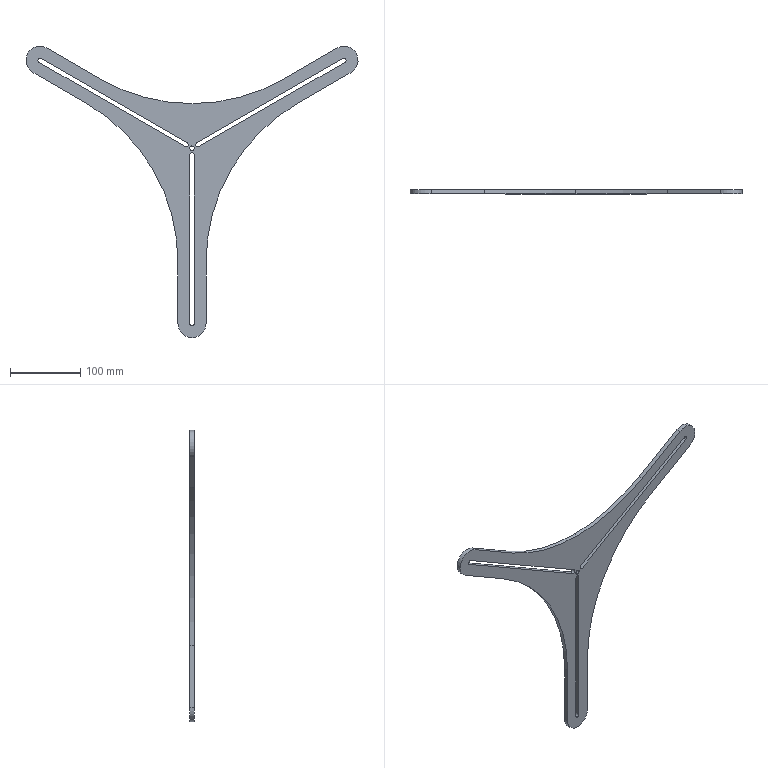Part | SolidWorks | features Extrusion 1 | 1 solid | 33 faces | box 472.147 x 6 x 414.25 mm | volume 225588 mm3 | cylinder 19 | plane 14 | commonest cylinder face diameters 6 x9 40 x4 520 x4 6.2 x2
STEP:
#1=CARTESIAN_POINT('',(15.557,6.,-256.75));
#2=VERTEX_POINT('',#1);
#3=CARTESIAN_POINT('',(12.557,6.,-259.75));
#4=VERTEX_POINT('',#3);
#5=CARTESIAN_POINT('',(12.557,6.,-256.75));
#6=DIRECTION('',(0.,1.,0.));
#7=DIRECTION('',(0.,0.,1.));
#8=AXIS2_PLACEMENT_3D('',#5,#6,#7);
#9=CIRCLE('',#8,3.);
#10=EDGE_CURVE('',#2,#4,#9,.T.);
#11=ORIENTED_EDGE('',*,*,#10,.T.);
#12=CARTESIAN_POINT('',(12.557,0.,-259.75));
#13=VERTEX_POINT('',#12);
#14=CARTESIAN_POINT('',(12.557,6.,-259.75));
#15=DIRECTION('',(0.,-1.,0.));
#16=VECTOR('',#15,1000.);
#17=LINE('',#14,#16);
#18=EDGE_CURVE('',#4,#13,#17,.T.);
#19=ORIENTED_EDGE('',*,*,#18,.T.);
#20=CARTESIAN_POINT('',(15.557,0.,-256.75));
#21=VERTEX_POINT('',#20);
#22=CARTESIAN_POINT('',(12.557,0.,-256.75));
#23=DIRECTION('',(0.,1.,0.));
#24=DIRECTION('',(0.,0.,1.));
#25=AXIS2_PLACEMENT_3D('',#22,#23,#24);
#26=CIRCLE('',#25,3.);
#27=EDGE_CURVE('',#21,#13,#26,.T.);
#28=ORIENTED_EDGE('',*,*,#27,.F.);
#29=CARTESIAN_POINT('',(15.557,6.,-256.75));
#30=DIRECTION('',(0.,-1.,0.));
#31=VECTOR('',#30,1000.);
#32=LINE('',#29,#31);
#33=EDGE_CURVE('',#2,#21,#32,.T.);
#34=ORIENTED_EDGE('',*,*,#33,.F.);
#35=EDGE_LOOP('',(#11,#19,#28,#34));
#36=FACE_OUTER_BOUND('',#35,.T.);
#37=CARTESIAN_POINT('',(12.557,6.,-256.75));
#38=DIRECTION('',(0.,-1.,0.));
#39=DIRECTION('',(0.,0.,-1.));
#40=AXIS2_PLACEMENT_3D('',#37,#38,#39);
#41=CYLINDRICAL_SURFACE('',#40,3.);
#42=ADVANCED_FACE('',(#36),#41,.F.);
#43=CARTESIAN_POINT('',(22.285,6.,-5.098));
#44=VERTEX_POINT('',#43);
#45=CARTESIAN_POINT('',(20.785,6.,-5.5));
#46=VERTEX_POINT('',#45);
#47=CARTESIAN_POINT('',(20.785,6.,-2.5));
#48=DIRECTION('',(0.,1.,0.));
#49=DIRECTION('',(0.,0.,1.));
#50=AXIS2_PLACEMENT_3D('',#47,#48,#49);
#51=CIRCLE('',#50,3.);
#52=EDGE_CURVE('',#44,#46,#51,.T.);
#53=ORIENTED_EDGE('',*,*,#52,.T.);
#54=CARTESIAN_POINT('',(20.785,0.,-5.5));
#55=VERTEX_POINT('',#54);
#56=CARTESIAN_POINT('',(20.785,6.,-5.5));
#57=DIRECTION('',(0.,-1.,0.));
#58=VECTOR('',#57,1000.);
#59=LINE('',#56,#58);
#60=EDGE_CURVE('',#46,#55,#59,.T.);
#61=ORIENTED_EDGE('',*,*,#60,.T.);
#62=CARTESIAN_POINT('',(22.285,0.,-5.098));
#63=VERTEX_POINT('',#62);
#64=CARTESIAN_POINT('',(20.785,0.,-2.5));
#65=DIRECTION('',(0.,1.,0.));
#66=DIRECTION('',(0.,0.,1.));
#67=AXIS2_PLACEMENT_3D('',#64,#65,#66);
#68=CIRCLE('',#67,3.);
#69=EDGE_CURVE('',#63,#55,#68,.T.);
#70=ORIENTED_EDGE('',*,*,#69,.F.);
#71=CARTESIAN_POINT('',(22.285,6.,-5.098));
#72=DIRECTION('',(0.,-1.,0.));
#73=VECTOR('',#72,1000.);
#74=LINE('',#71,#73);
#75=EDGE_CURVE('',#44,#63,#74,.T.);
#76=ORIENTED_EDGE('',*,*,#75,.F.);
#77=EDGE_LOOP('',(#53,#61,#70,#76));
#78=FACE_OUTER_BOUND('',#77,.T.);
#79=CARTESIAN_POINT('',(20.785,6.,-2.5));
#80=DIRECTION('',(0.,-1.,0.));
#81=DIRECTION('',(0.,0.,-1.));
#82=AXIS2_PLACEMENT_3D('',#79,#80,#81);
#83=CYLINDRICAL_SURFACE('',#82,3.);
#84=ADVANCED_FACE('',(#78),#83,.F.);
#85=CARTESIAN_POINT('',(5.83,6.,0.09808));
#86=VERTEX_POINT('',#85);
#87=CARTESIAN_POINT('',(4.33,6.,-5.5));
#88=VERTEX_POINT('',#87);
#89=CARTESIAN_POINT('',(4.33,6.,-2.5));
#90=DIRECTION('',(0.,1.,0.));
#91=DIRECTION('',(0.,0.,1.));
#92=AXIS2_PLACEMENT_3D('',#89,#90,#91);
#93=CIRCLE('',#92,3.);
#94=EDGE_CURVE('',#86,#88,#93,.T.);
#95=ORIENTED_EDGE('',*,*,#94,.T.);
#96=CARTESIAN_POINT('',(4.33,0.,-5.5));
#97=VERTEX_POINT('',#96);
#98=CARTESIAN_POINT('',(4.33,6.,-5.5));
#99=DIRECTION('',(0.,-1.,0.));
#100=VECTOR('',#99,1000.);
#101=LINE('',#98,#100);
#102=EDGE_CURVE('',#88,#97,#101,.T.);
#103=ORIENTED_EDGE('',*,*,#102,.T.);
#104=CARTESIAN_POINT('',(5.83,0.,0.09808));
#105=VERTEX_POINT('',#104);
#106=CARTESIAN_POINT('',(4.33,0.,-2.5));
#107=DIRECTION('',(0.,1.,0.));
#108=DIRECTION('',(0.,0.,1.));
#109=AXIS2_PLACEMENT_3D('',#106,#107,#108);
#110=CIRCLE('',#109,3.);
#111=EDGE_CURVE('',#105,#97,#110,.T.);
#112=ORIENTED_EDGE('',*,*,#111,.F.);
#113=CARTESIAN_POINT('',(5.83,6.,0.09808));
#114=DIRECTION('',(0.,-1.,0.));
#115=VECTOR('',#114,1000.);
#116=LINE('',#113,#115);
#117=EDGE_CURVE('',#86,#105,#116,.T.);
#118=ORIENTED_EDGE('',*,*,#117,.F.);
#119=EDGE_LOOP('',(#95,#103,#112,#118));
#120=FACE_OUTER_BOUND('',#119,.T.);
#121=CARTESIAN_POINT('',(4.33,6.,-2.5));
#122=DIRECTION('',(0.,-1.,0.));
#123=DIRECTION('',(0.,0.,-1.));
#124=AXIS2_PLACEMENT_3D('',#121,#122,#123);
#125=CYLINDRICAL_SURFACE('',#124,3.);
#126=ADVANCED_FACE('',(#120),#125,.F.);
#127=CARTESIAN_POINT('',(12.557,6.,-10.35));
#128=VERTEX_POINT('',#127);
#129=CARTESIAN_POINT('',(12.557,6.,-4.15));
#130=VERTEX_POINT('',#129);
#131=CARTESIAN_POINT('',(12.557,6.,-7.25));
#132=DIRECTION('',(0.,1.,0.));
#133=DIRECTION('',(0.,0.,1.));
#134=AXIS2_PLACEMENT_3D('',#131,#132,#133);
#135=CIRCLE('',#134,3.1);
#136=EDGE_CURVE('',#128,#130,#135,.T.);
#137=ORIENTED_EDGE('',*,*,#136,.T.);
#138=CARTESIAN_POINT('',(12.557,0.,-4.15));
#139=VERTEX_POINT('',#138);
#140=CARTESIAN_POINT('',(12.557,6.,-4.15));
#141=DIRECTION('',(0.,-1.,0.));
#142=VECTOR('',#141,1000.);
#143=LINE('',#140,#142);
#144=EDGE_CURVE('',#130,#139,#143,.T.);
#145=ORIENTED_EDGE('',*,*,#144,.T.);
#146=CARTESIAN_POINT('',(12.557,0.,-10.35));
#147=VERTEX_POINT('',#146);
#148=CARTESIAN_POINT('',(12.557,0.,-7.25));
#149=DIRECTION('',(0.,1.,0.));
#150=DIRECTION('',(0.,0.,1.));
#151=AXIS2_PLACEMENT_3D('',#148,#149,#150);
#152=CIRCLE('',#151,3.1);
#153=EDGE_CURVE('',#147,#139,#152,.T.);
#154=ORIENTED_EDGE('',*,*,#153,.F.);
#155=CARTESIAN_POINT('',(12.557,6.,-10.35));
#156=DIRECTION('',(0.,-1.,0.));
#157=VECTOR('',#156,1000.);
#158=LINE('',#155,#157);
#159=EDGE_CURVE('',#128,#147,#158,.T.);
#160=ORIENTED_EDGE('',*,*,#159,.F.);
#161=EDGE_LOOP('',(#137,#145,#154,#160));
#162=FACE_OUTER_BOUND('',#161,.T.);
#163=CARTESIAN_POINT('',(12.557,6.,-7.25));
#164=DIRECTION('',(0.,-1.,0.));
#165=DIRECTION('',(0.,0.,-1.));
#166=AXIS2_PLACEMENT_3D('',#163,#164,#165);
#167=CYLINDRICAL_SURFACE('',#166,3.1);
#168=ADVANCED_FACE('',(#162),#167,.F.);
#169=CARTESIAN_POINT('',(12.557,6.,56.066));
#170=VERTEX_POINT('',#169);
#171=CARTESIAN_POINT('',(142.557,6.,90.9));
#172=VERTEX_POINT('',#171);
#173=CARTESIAN_POINT('',(12.557,6.,316.066));
#174=DIRECTION('',(0.,-1.,0.));
#175=DIRECTION('',(0.,0.,-1.));
#176=AXIS2_PLACEMENT_3D('',#173,#174,#175);
#177=CIRCLE('',#176,260.);
#178=EDGE_CURVE('',#170,#172,#177,.T.);
#179=ORIENTED_EDGE('',*,*,#178,.F.);
#180=CARTESIAN_POINT('',(12.557,0.,56.066));
#181=VERTEX_POINT('',#180);
#182=CARTESIAN_POINT('',(12.557,6.,56.066));
#183=DIRECTION('',(0.,-1.,0.));
#184=VECTOR('',#183,1000.);
#185=LINE('',#182,#184);
#186=EDGE_CURVE('',#170,#181,#185,.T.);
#187=ORIENTED_EDGE('',*,*,#186,.T.);
#188=CARTESIAN_POINT('',(142.557,0.,90.9));
#189=VERTEX_POINT('',#188);
#190=CARTESIAN_POINT('',(12.557,0.,316.066));
#191=DIRECTION('',(0.,-1.,0.));
#192=DIRECTION('',(0.,0.,-1.));
#193=AXIS2_PLACEMENT_3D('',#190,#191,#192);
#194=CIRCLE('',#193,260.);
#195=EDGE_CURVE('',#181,#189,#194,.T.);
#196=ORIENTED_EDGE('',*,*,#195,.T.);
#197=CARTESIAN_POINT('',(142.557,6.,90.9));
#198=DIRECTION('',(0.,-1.,0.));
#199=VECTOR('',#198,1000.);
#200=LINE('',#197,#199);
#201=EDGE_CURVE('',#172,#189,#200,.T.);
#202=ORIENTED_EDGE('',*,*,#201,.F.);
#203=EDGE_LOOP('',(#179,#187,#196,#202));
#204=FACE_OUTER_BOUND('',#203,.T.);
#205=CARTESIAN_POINT('',(12.557,6.,316.066));
#206=DIRECTION('',(0.,-1.,0.));
#207=DIRECTION('',(0.,0.,-1.));
#208=AXIS2_PLACEMENT_3D('',#205,#206,#207);
#209=CYLINDRICAL_SURFACE('',#208,260.);
#210=ADVANCED_FACE('',(#204),#209,.F.);
#211=CARTESIAN_POINT('',(12.557,6.,-276.75));
#212=VERTEX_POINT('',#211);
#213=CARTESIAN_POINT('',(-7.443,6.,-256.75));
#214=VERTEX_POINT('',#213);
#215=CARTESIAN_POINT('',(12.557,6.,-256.75));
#216=DIRECTION('',(0.,1.,0.));
#217=DIRECTION('',(0.,0.,-1.));
#218=AXIS2_PLACEMENT_3D('',#215,#216,#217);
#219=CIRCLE('',#218,20.);
#220=EDGE_CURVE('',#212,#214,#219,.T.);
#221=ORIENTED_EDGE('',*,*,#220,.F.);
#222=CARTESIAN_POINT('',(12.557,0.,-276.75));
#223=VERTEX_POINT('',#222);
#224=CARTESIAN_POINT('',(12.557,6.,-276.75));
#225=DIRECTION('',(0.,-1.,0.));
#226=VECTOR('',#225,1000.);
#227=LINE('',#224,#226);
#228=EDGE_CURVE('',#212,#223,#227,.T.);
#229=ORIENTED_EDGE('',*,*,#228,.T.);
#230=CARTESIAN_POINT('',(-7.443,0.,-256.75));
#231=VERTEX_POINT('',#230);
#232=CARTESIAN_POINT('',(12.557,0.,-256.75));
#233=DIRECTION('',(0.,1.,0.));
#234=DIRECTION('',(0.,0.,-1.));
#235=AXIS2_PLACEMENT_3D('',#232,#233,#234);
#236=CIRCLE('',#235,20.);
#237=EDGE_CURVE('',#223,#231,#236,.T.);
#238=ORIENTED_EDGE('',*,*,#237,.T.);
#239=CARTESIAN_POINT('',(-7.443,6.,-256.75));
#240=DIRECTION('',(0.,-1.,0.));
#241=VECTOR('',#240,1000.);
#242=LINE('',#239,#241);
#243=EDGE_CURVE('',#214,#231,#242,.T.);
#244=ORIENTED_EDGE('',*,*,#243,.F.);
#245=EDGE_LOOP('',(#221,#229,#238,#244));
#246=FACE_OUTER_BOUND('',#245,.T.);
#247=CARTESIAN_POINT('',(12.557,6.,-256.75));
#248=DIRECTION('',(0.,-1.,0.));
#249=DIRECTION('',(0.,0.,-1.));
#250=AXIS2_PLACEMENT_3D('',#247,#248,#249);
#251=CYLINDRICAL_SURFACE('',#250,20.);
#252=ADVANCED_FACE('',(#246),#251,.T.);
#253=ORIENTED_EDGE('',*,*,#52,.F.);
#254=CARTESIAN_POINT('',(230.131,6.,114.902));
#255=VERTEX_POINT('',#254);
#256=CARTESIAN_POINT('',(22.285,6.,-5.098));
#257=DIRECTION('',(-0.866,0.,-0.5));
#258=VECTOR('',#257,1000.);
#259=LINE('',#256,#258);
#260=EDGE_CURVE('',#255,#44,#259,.T.);
#261=ORIENTED_EDGE('',*,*,#260,.F.);
#262=CARTESIAN_POINT('',(227.131,6.,120.098));
#263=VERTEX_POINT('',#262);
#264=CARTESIAN_POINT('',(228.631,6.,117.5));
#265=DIRECTION('',(0.,1.,0.));
#266=DIRECTION('',(0.,0.,1.));
#267=AXIS2_PLACEMENT_3D('',#264,#265,#266);
#268=CIRCLE('',#267,3.);
#269=EDGE_CURVE('',#263,#255,#268,.T.);
#270=ORIENTED_EDGE('',*,*,#269,.F.);
#271=CARTESIAN_POINT('',(19.285,6.,0.09808));
#272=VERTEX_POINT('',#271);
#273=CARTESIAN_POINT('',(19.285,6.,0.09808));
#274=DIRECTION('',(0.866,0.,0.5));
#275=VECTOR('',#274,1000.);
#276=LINE('',#273,#275);
#277=EDGE_CURVE('',#272,#263,#276,.T.);
#278=ORIENTED_EDGE('',*,*,#277,.F.);
#279=CARTESIAN_POINT('',(20.785,6.,-2.5));
#280=DIRECTION('',(0.,1.,0.));
#281=DIRECTION('',(0.,0.,1.));
#282=AXIS2_PLACEMENT_3D('',#279,#280,#281);
#283=CIRCLE('',#282,3.);
#284=EDGE_CURVE('',#46,#272,#283,.T.);
#285=ORIENTED_EDGE('',*,*,#284,.F.);
#286=EDGE_LOOP('',(#253,#261,#270,#278,#285));
#287=FACE_BOUND('',#286,.T.);
#288=ORIENTED_EDGE('',*,*,#136,.F.);
#289=CARTESIAN_POINT('',(12.557,6.,-7.25));
#290=DIRECTION('',(0.,1.,0.));
#291=DIRECTION('',(0.,0.,1.));
#292=AXIS2_PLACEMENT_3D('',#289,#290,#291);
#293=CIRCLE('',#292,3.1);
#294=EDGE_CURVE('',#130,#128,#293,.T.);
#295=ORIENTED_EDGE('',*,*,#294,.F.);
#296=EDGE_LOOP('',(#288,#295));
#297=FACE_BOUND('',#296,.T.);
#298=CARTESIAN_POINT('',(32.557,6.,-256.75));
#299=VERTEX_POINT('',#298);
#300=CARTESIAN_POINT('',(12.557,6.,-256.75));
#301=DIRECTION('',(0.,1.,0.));
#302=DIRECTION('',(0.,0.,-1.));
#303=AXIS2_PLACEMENT_3D('',#300,#301,#302);
#304=CIRCLE('',#303,20.);
#305=EDGE_CURVE('',#299,#212,#304,.T.);
#306=ORIENTED_EDGE('',*,*,#305,.T.);
#307=ORIENTED_EDGE('',*,*,#220,.T.);
#308=CARTESIAN_POINT('',(-7.443,6.,-168.908));
#309=VERTEX_POINT('',#308);
#310=CARTESIAN_POINT('',(-7.443,6.,-168.908));
#311=DIRECTION('',(0.,0.,1.));
#312=VECTOR('',#311,1000.);
#313=LINE('',#310,#312);
#314=EDGE_CURVE('',#214,#309,#313,.T.);
#315=ORIENTED_EDGE('',*,*,#314,.T.);
#316=CARTESIAN_POINT('',(-137.443,6.,56.259));
#317=VERTEX_POINT('',#316);
#318=CARTESIAN_POINT('',(-267.443,6.,-168.908));
#319=DIRECTION('',(0.,-1.,0.));
#320=DIRECTION('',(0.,0.,-1.));
#321=AXIS2_PLACEMENT_3D('',#318,#319,#320);
#322=CIRCLE('',#321,260.);
#323=EDGE_CURVE('',#309,#317,#322,.T.);
#324=ORIENTED_EDGE('',*,*,#323,.T.);
#325=CARTESIAN_POINT('',(-213.516,6.,100.179));
#326=VERTEX_POINT('',#325);
#327=CARTESIAN_POINT('',(-137.443,6.,56.259));
#328=DIRECTION('',(-0.866,0.,0.5));
#329=VECTOR('',#328,1000.);
#330=LINE('',#327,#329);
#331=EDGE_CURVE('',#317,#326,#330,.T.);
#332=ORIENTED_EDGE('',*,*,#331,.T.);
#333=CARTESIAN_POINT('',(-193.516,6.,134.821));
#334=VERTEX_POINT('',#333);
#335=CARTESIAN_POINT('',(-203.516,6.,117.5));
#336=DIRECTION('',(0.,1.,0.));
#337=DIRECTION('',(0.,0.,1.));
#338=AXIS2_PLACEMENT_3D('',#335,#336,#337);
#339=CIRCLE('',#338,20.);
#340=EDGE_CURVE('',#326,#334,#339,.T.);
#341=ORIENTED_EDGE('',*,*,#340,.T.);
#342=CARTESIAN_POINT('',(-117.443,6.,90.9));
#343=VERTEX_POINT('',#342);
#344=CARTESIAN_POINT('',(-117.443,6.,90.9));
#345=DIRECTION('',(0.866,0.,-0.5));
#346=VECTOR('',#345,1000.);
#347=LINE('',#344,#346);
#348=EDGE_CURVE('',#334,#343,#347,.T.);
#349=ORIENTED_EDGE('',*,*,#348,.T.);
#350=CARTESIAN_POINT('',(12.557,6.,316.066));
#351=DIRECTION('',(0.,-1.,0.));
#352=DIRECTION('',(0.,0.,-1.));
#353=AXIS2_PLACEMENT_3D('',#350,#351,#352);
#354=CIRCLE('',#353,260.);
#355=EDGE_CURVE('',#343,#170,#354,.T.);
#356=ORIENTED_EDGE('',*,*,#355,.T.);
#357=ORIENTED_EDGE('',*,*,#178,.T.);
#358=CARTESIAN_POINT('',(218.631,6.,134.821));
#359=VERTEX_POINT('',#358);
#360=CARTESIAN_POINT('',(142.557,6.,90.9));
#361=DIRECTION('',(0.866,0.,0.5));
#362=VECTOR('',#361,1000.);
#363=LINE('',#360,#362);
#364=EDGE_CURVE('',#172,#359,#363,.T.);
#365=ORIENTED_EDGE('',*,*,#364,.T.);
#366=CARTESIAN_POINT('',(238.631,6.,100.179));
#367=VERTEX_POINT('',#366);
#368=CARTESIAN_POINT('',(228.631,6.,117.5));
#369=DIRECTION('',(0.,1.,0.));
#370=DIRECTION('',(0.,0.,-1.));
#371=AXIS2_PLACEMENT_3D('',#368,#369,#370);
#372=CIRCLE('',#371,20.);
#373=EDGE_CURVE('',#359,#367,#372,.T.);
#374=ORIENTED_EDGE('',*,*,#373,.T.);
#375=CARTESIAN_POINT('',(162.557,6.,56.259));
#376=VERTEX_POINT('',#375);
#377=CARTESIAN_POINT('',(162.557,6.,56.259));
#378=DIRECTION('',(-0.866,0.,-0.5));
#379=VECTOR('',#378,1000.);
#380=LINE('',#377,#379);
#381=EDGE_CURVE('',#367,#376,#380,.T.);
#382=ORIENTED_EDGE('',*,*,#381,.T.);
#383=CARTESIAN_POINT('',(32.557,6.,-168.908));
#384=VERTEX_POINT('',#383);
#385=CARTESIAN_POINT('',(292.557,6.,-168.908));
#386=DIRECTION('',(0.,-1.,0.));
#387=DIRECTION('',(0.,0.,-1.));
#388=AXIS2_PLACEMENT_3D('',#385,#386,#387);
#389=CIRCLE('',#388,260.);
#390=EDGE_CURVE('',#376,#384,#389,.T.);
#391=ORIENTED_EDGE('',*,*,#390,.T.);
#392=CARTESIAN_POINT('',(32.557,6.,-168.908));
#393=DIRECTION('',(0.,0.,-1.));
#394=VECTOR('',#393,1000.);
#395=LINE('',#392,#394);
#396=EDGE_CURVE('',#384,#299,#395,.T.);
#397=ORIENTED_EDGE('',*,*,#396,.T.);
#398=EDGE_LOOP('',(#306,#307,#315,#324,#332,#341,#349,#356,#357,#365,#374,#382,#391,#397));
#399=FACE_OUTER_BOUND('',#398,.T.);
#400=ORIENTED_EDGE('',*,*,#94,.F.);
#401=CARTESIAN_POINT('',(-202.016,6.,120.098));
#402=VERTEX_POINT('',#401);
#403=CARTESIAN_POINT('',(5.83,6.,0.09808));
#404=DIRECTION('',(0.866,0.,-0.5));
#405=VECTOR('',#404,1000.);
#406=LINE('',#403,#405);
#407=EDGE_CURVE('',#402,#86,#406,.T.);
#408=ORIENTED_EDGE('',*,*,#407,.F.);
#409=CARTESIAN_POINT('',(-205.016,6.,114.902));
#410=VERTEX_POINT('',#409);
#411=CARTESIAN_POINT('',(-203.516,6.,117.5));
#412=DIRECTION('',(0.,1.,0.));
#413=DIRECTION('',(0.,0.,1.));
#414=AXIS2_PLACEMENT_3D('',#411,#412,#413);
#415=CIRCLE('',#414,3.);
#416=EDGE_CURVE('',#410,#402,#415,.T.);
#417=ORIENTED_EDGE('',*,*,#416,.F.);
#418=CARTESIAN_POINT('',(2.83,6.,-5.098));
#419=VERTEX_POINT('',#418);
#420=CARTESIAN_POINT('',(2.83,6.,-5.098));
#421=DIRECTION('',(-0.866,0.,0.5));
#422=VECTOR('',#421,1000.);
#423=LINE('',#420,#422);
#424=EDGE_CURVE('',#419,#410,#423,.T.);
#425=ORIENTED_EDGE('',*,*,#424,.F.);
#426=CARTESIAN_POINT('',(4.33,6.,-2.5));
#427=DIRECTION('',(0.,1.,0.));
#428=DIRECTION('',(0.,0.,1.));
#429=AXIS2_PLACEMENT_3D('',#426,#427,#428);
#430=CIRCLE('',#429,3.);
#431=EDGE_CURVE('',#88,#419,#430,.T.);
#432=ORIENTED_EDGE('',*,*,#431,.F.);
#433=EDGE_LOOP('',(#400,#408,#417,#425,#432));
#434=FACE_BOUND('',#433,.T.);
#435=CARTESIAN_POINT('',(9.557,6.,-16.75));
#436=VERTEX_POINT('',#435);
#437=CARTESIAN_POINT('',(15.557,6.,-16.75));
#438=VERTEX_POINT('',#437);
#439=CARTESIAN_POINT('',(12.557,6.,-16.75));
#440=DIRECTION('',(0.,1.,0.));
#441=DIRECTION('',(0.,0.,1.));
#442=AXIS2_PLACEMENT_3D('',#439,#440,#441);
#443=CIRCLE('',#442,3.);
#444=EDGE_CURVE('',#436,#438,#443,.T.);
#445=ORIENTED_EDGE('',*,*,#444,.F.);
#446=CARTESIAN_POINT('',(9.557,6.,-256.75));
#447=VERTEX_POINT('',#446);
#448=CARTESIAN_POINT('',(9.557,6.,-16.75));
#449=DIRECTION('',(0.,0.,1.));
#450=VECTOR('',#449,1000.);
#451=LINE('',#448,#450);
#452=EDGE_CURVE('',#447,#436,#451,.T.);
#453=ORIENTED_EDGE('',*,*,#452,.F.);
#454=CARTESIAN_POINT('',(12.557,6.,-256.75));
#455=DIRECTION('',(0.,1.,0.));
#456=DIRECTION('',(0.,0.,1.));
#457=AXIS2_PLACEMENT_3D('',#454,#455,#456);
#458=CIRCLE('',#457,3.);
#459=EDGE_CURVE('',#4,#447,#458,.T.);
#460=ORIENTED_EDGE('',*,*,#459,.F.);
#461=ORIENTED_EDGE('',*,*,#10,.F.);
#462=CARTESIAN_POINT('',(15.557,6.,-16.75));
#463=DIRECTION('',(0.,0.,-1.));
#464=VECTOR('',#463,1000.);
#465=LINE('',#462,#464);
#466=EDGE_CURVE('',#438,#2,#465,.T.);
#467=ORIENTED_EDGE('',*,*,#466,.F.);
#468=EDGE_LOOP('',(#445,#453,#460,#461,#467));
#469=FACE_BOUND('',#468,.T.);
#470=CARTESIAN_POINT('',(12.557,6.,-256.75));
#471=DIRECTION('',(0.,-1.,0.));
#472=DIRECTION('',(0.,0.,-1.));
#473=AXIS2_PLACEMENT_3D('',#470,#471,#472);
#474=PLANE('',#473);
#475=ADVANCED_FACE('',(#287,#297,#399,#434,#469),#474,.F.);
#476=CARTESIAN_POINT('',(230.131,0.,114.902));
#477=VERTEX_POINT('',#476);
#478=CARTESIAN_POINT('',(22.285,0.,-5.098));
#479=DIRECTION('',(-0.866,0.,-0.5));
#480=VECTOR('',#479,1000.);
#481=LINE('',#478,#480);
#482=EDGE_CURVE('',#477,#63,#481,.T.);
#483=ORIENTED_EDGE('',*,*,#482,.T.);
#484=ORIENTED_EDGE('',*,*,#69,.T.);
#485=CARTESIAN_POINT('',(19.285,0.,0.09808));
#486=VERTEX_POINT('',#485);
#487=CARTESIAN_POINT('',(20.785,0.,-2.5));
#488=DIRECTION('',(0.,1.,0.));
#489=DIRECTION('',(0.,0.,1.));
#490=AXIS2_PLACEMENT_3D('',#487,#488,#489);
#491=CIRCLE('',#490,3.);
#492=EDGE_CURVE('',#55,#486,#491,.T.);
#493=ORIENTED_EDGE('',*,*,#492,.T.);
#494=CARTESIAN_POINT('',(227.131,0.,120.098));
#495=VERTEX_POINT('',#494);
#496=CARTESIAN_POINT('',(19.285,0.,0.09808));
#497=DIRECTION('',(0.866,0.,0.5));
#498=VECTOR('',#497,1000.);
#499=LINE('',#496,#498);
#500=EDGE_CURVE('',#486,#495,#499,.T.);
#501=ORIENTED_EDGE('',*,*,#500,.T.);
#502=CARTESIAN_POINT('',(228.631,0.,117.5));
#503=DIRECTION('',(0.,1.,0.));
#504=DIRECTION('',(0.,0.,1.));
#505=AXIS2_PLACEMENT_3D('',#502,#503,#504);
#506=CIRCLE('',#505,3.);
#507=EDGE_CURVE('',#495,#477,#506,.T.);
#508=ORIENTED_EDGE('',*,*,#507,.T.);
#509=EDGE_LOOP('',(#483,#484,#493,#501,#508));
#510=FACE_BOUND('',#509,.T.);
#511=ORIENTED_EDGE('',*,*,#153,.T.);
#512=CARTESIAN_POINT('',(12.557,0.,-7.25));
#513=DIRECTION('',(0.,1.,0.));
#514=DIRECTION('',(0.,0.,1.));
#515=AXIS2_PLACEMENT_3D('',#512,#513,#514);
#516=CIRCLE('',#515,3.1);
#517=EDGE_CURVE('',#139,#147,#516,.T.);
#518=ORIENTED_EDGE('',*,*,#517,.T.);
#519=EDGE_LOOP('',(#511,#518));
#520=FACE_BOUND('',#519,.T.);
#521=CARTESIAN_POINT('',(32.557,0.,-256.75));
#522=VERTEX_POINT('',#521);
#523=CARTESIAN_POINT('',(12.557,0.,-256.75));
#524=DIRECTION('',(0.,1.,0.));
#525=DIRECTION('',(0.,0.,-1.));
#526=AXIS2_PLACEMENT_3D('',#523,#524,#525);
#527=CIRCLE('',#526,20.);
#528=EDGE_CURVE('',#522,#223,#527,.T.);
#529=ORIENTED_EDGE('',*,*,#528,.F.);
#530=CARTESIAN_POINT('',(32.557,0.,-168.908));
#531=VERTEX_POINT('',#530);
#532=CARTESIAN_POINT('',(32.557,0.,-168.908));
#533=DIRECTION('',(0.,0.,-1.));
#534=VECTOR('',#533,1000.);
#535=LINE('',#532,#534);
#536=EDGE_CURVE('',#531,#522,#535,.T.);
#537=ORIENTED_EDGE('',*,*,#536,.F.);
#538=CARTESIAN_POINT('',(162.557,0.,56.259));
#539=VERTEX_POINT('',#538);
#540=CARTESIAN_POINT('',(292.557,0.,-168.908));
#541=DIRECTION('',(0.,-1.,0.));
#542=DIRECTION('',(0.,0.,-1.));
#543=AXIS2_PLACEMENT_3D('',#540,#541,#542);
#544=CIRCLE('',#543,260.);
#545=EDGE_CURVE('',#539,#531,#544,.T.);
#546=ORIENTED_EDGE('',*,*,#545,.F.);
#547=CARTESIAN_POINT('',(238.631,0.,100.179));
#548=VERTEX_POINT('',#547);
#549=CARTESIAN_POINT('',(162.557,0.,56.259));
#550=DIRECTION('',(-0.866,0.,-0.5));
#551=VECTOR('',#550,1000.);
#552=LINE('',#549,#551);
#553=EDGE_CURVE('',#548,#539,#552,.T.);
#554=ORIENTED_EDGE('',*,*,#553,.F.);
#555=CARTESIAN_POINT('',(218.631,0.,134.821));
#556=VERTEX_POINT('',#555);
#557=CARTESIAN_POINT('',(228.631,0.,117.5));
#558=DIRECTION('',(0.,1.,0.));
#559=DIRECTION('',(0.,0.,-1.));
#560=AXIS2_PLACEMENT_3D('',#557,#558,#559);
#561=CIRCLE('',#560,20.);
#562=EDGE_CURVE('',#556,#548,#561,.T.);
#563=ORIENTED_EDGE('',*,*,#562,.F.);
#564=CARTESIAN_POINT('',(142.557,0.,90.9));
#565=DIRECTION('',(0.866,0.,0.5));
#566=VECTOR('',#565,1000.);
#567=LINE('',#564,#566);
#568=EDGE_CURVE('',#189,#556,#567,.T.);
#569=ORIENTED_EDGE('',*,*,#568,.F.);
#570=ORIENTED_EDGE('',*,*,#195,.F.);
#571=CARTESIAN_POINT('',(-117.443,0.,90.9));
#572=VERTEX_POINT('',#571);
#573=CARTESIAN_POINT('',(12.557,0.,316.066));
#574=DIRECTION('',(0.,-1.,0.));
#575=DIRECTION('',(0.,0.,-1.));
#576=AXIS2_PLACEMENT_3D('',#573,#574,#575);
#577=CIRCLE('',#576,260.);
#578=EDGE_CURVE('',#572,#181,#577,.T.);
#579=ORIENTED_EDGE('',*,*,#578,.F.);
#580=CARTESIAN_POINT('',(-193.516,0.,134.821));
#581=VERTEX_POINT('',#580);
#582=CARTESIAN_POINT('',(-117.443,0.,90.9));
#583=DIRECTION('',(0.866,0.,-0.5));
#584=VECTOR('',#583,1000.);
#585=LINE('',#582,#584);
#586=EDGE_CURVE('',#581,#572,#585,.T.);
#587=ORIENTED_EDGE('',*,*,#586,.F.);
#588=CARTESIAN_POINT('',(-213.516,0.,100.179));
#589=VERTEX_POINT('',#588);
#590=CARTESIAN_POINT('',(-203.516,0.,117.5));
#591=DIRECTION('',(0.,1.,0.));
#592=DIRECTION('',(0.,0.,1.));
#593=AXIS2_PLACEMENT_3D('',#590,#591,#592);
#594=CIRCLE('',#593,20.);
#595=EDGE_CURVE('',#589,#581,#594,.T.);
#596=ORIENTED_EDGE('',*,*,#595,.F.);
#597=CARTESIAN_POINT('',(-137.443,0.,56.259));
#598=VERTEX_POINT('',#597);
#599=CARTESIAN_POINT('',(-137.443,0.,56.259));
#600=DIRECTION('',(-0.866,0.,0.5));
#601=VECTOR('',#600,1000.);
#602=LINE('',#599,#601);
#603=EDGE_CURVE('',#598,#589,#602,.T.);
#604=ORIENTED_EDGE('',*,*,#603,.F.);
#605=CARTESIAN_POINT('',(-7.443,0.,-168.908));
#606=VERTEX_POINT('',#605);
#607=CARTESIAN_POINT('',(-267.443,0.,-168.908));
#608=DIRECTION('',(0.,-1.,0.));
#609=DIRECTION('',(0.,0.,-1.));
#610=AXIS2_PLACEMENT_3D('',#607,#608,#609);
#611=CIRCLE('',#610,260.);
#612=EDGE_CURVE('',#606,#598,#611,.T.);
#613=ORIENTED_EDGE('',*,*,#612,.F.);
#614=CARTESIAN_POINT('',(-7.443,0.,-168.908));
#615=DIRECTION('',(0.,0.,1.));
#616=VECTOR('',#615,1000.);
#617=LINE('',#614,#616);
#618=EDGE_CURVE('',#231,#606,#617,.T.);
#619=ORIENTED_EDGE('',*,*,#618,.F.);
#620=ORIENTED_EDGE('',*,*,#237,.F.);
#621=EDGE_LOOP('',(#529,#537,#546,#554,#563,#569,#570,#579,#587,#596,#604,#613,#619,#620));
#622=FACE_OUTER_BOUND('',#621,.T.);
#623=CARTESIAN_POINT('',(-202.016,0.,120.098));
#624=VERTEX_POINT('',#623);
#625=CARTESIAN_POINT('',(5.83,0.,0.09808));
#626=DIRECTION('',(0.866,0.,-0.5));
#627=VECTOR('',#626,1000.);
#628=LINE('',#625,#627);
#629=EDGE_CURVE('',#624,#105,#628,.T.);
#630=ORIENTED_EDGE('',*,*,#629,.T.);
#631=ORIENTED_EDGE('',*,*,#111,.T.);
#632=CARTESIAN_POINT('',(2.83,0.,-5.098));
#633=VERTEX_POINT('',#632);
#634=CARTESIAN_POINT('',(4.33,0.,-2.5));
#635=DIRECTION('',(0.,1.,0.));
#636=DIRECTION('',(0.,0.,1.));
#637=AXIS2_PLACEMENT_3D('',#634,#635,#636);
#638=CIRCLE('',#637,3.);
#639=EDGE_CURVE('',#97,#633,#638,.T.);
#640=ORIENTED_EDGE('',*,*,#639,.T.);
#641=CARTESIAN_POINT('',(-205.016,0.,114.902));
#642=VERTEX_POINT('',#641);
#643=CARTESIAN_POINT('',(2.83,0.,-5.098));
#644=DIRECTION('',(-0.866,0.,0.5));
#645=VECTOR('',#644,1000.);
#646=LINE('',#643,#645);
#647=EDGE_CURVE('',#633,#642,#646,.T.);
#648=ORIENTED_EDGE('',*,*,#647,.T.);
#649=CARTESIAN_POINT('',(-203.516,0.,117.5));
#650=DIRECTION('',(0.,1.,0.));
#651=DIRECTION('',(0.,0.,1.));
#652=AXIS2_PLACEMENT_3D('',#649,#650,#651);
#653=CIRCLE('',#652,3.);
#654=EDGE_CURVE('',#642,#624,#653,.T.);
#655=ORIENTED_EDGE('',*,*,#654,.T.);
#656=EDGE_LOOP('',(#630,#631,#640,#648,#655));
#657=FACE_BOUND('',#656,.T.);
#658=CARTESIAN_POINT('',(9.557,0.,-256.75));
#659=VERTEX_POINT('',#658);
#660=CARTESIAN_POINT('',(9.557,0.,-16.75));
#661=VERTEX_POINT('',#660);
#662=CARTESIAN_POINT('',(9.557,0.,-16.75));
#663=DIRECTION('',(0.,0.,1.));
#664=VECTOR('',#663,1000.);
#665=LINE('',#662,#664);
#666=EDGE_CURVE('',#659,#661,#665,.T.);
#667=ORIENTED_EDGE('',*,*,#666,.T.);
#668=CARTESIAN_POINT('',(15.557,0.,-16.75));
#669=VERTEX_POINT('',#668);
#670=CARTESIAN_POINT('',(12.557,0.,-16.75));
#671=DIRECTION('',(0.,1.,0.));
#672=DIRECTION('',(0.,0.,1.));
#673=AXIS2_PLACEMENT_3D('',#670,#671,#672);
#674=CIRCLE('',#673,3.);
#675=EDGE_CURVE('',#661,#669,#674,.T.);
#676=ORIENTED_EDGE('',*,*,#675,.T.);
#677=CARTESIAN_POINT('',(15.557,0.,-16.75));
#678=DIRECTION('',(0.,0.,-1.));
#679=VECTOR('',#678,1000.);
#680=LINE('',#677,#679);
#681=EDGE_CURVE('',#669,#21,#680,.T.);
#682=ORIENTED_EDGE('',*,*,#681,.T.);
#683=ORIENTED_EDGE('',*,*,#27,.T.);
#684=CARTESIAN_POINT('',(12.557,0.,-256.75));
#685=DIRECTION('',(0.,1.,0.));
#686=DIRECTION('',(0.,0.,1.));
#687=AXIS2_PLACEMENT_3D('',#684,#685,#686);
#688=CIRCLE('',#687,3.);
#689=EDGE_CURVE('',#13,#659,#688,.T.);
#690=ORIENTED_EDGE('',*,*,#689,.T.);
#691=EDGE_LOOP('',(#667,#676,#682,#683,#690));
#692=FACE_BOUND('',#691,.T.);
#693=CARTESIAN_POINT('',(12.557,0.,-256.75));
#694=DIRECTION('',(0.,-1.,0.));
#695=DIRECTION('',(0.,0.,-1.));
#696=AXIS2_PLACEMENT_3D('',#693,#694,#695);
#697=PLANE('',#696);
#698=ADVANCED_FACE('',(#510,#520,#622,#657,#692),#697,.T.);
#699=ORIENTED_EDGE('',*,*,#228,.F.);
#700=ORIENTED_EDGE('',*,*,#305,.F.);
#701=CARTESIAN_POINT('',(32.557,6.,-256.75));
#702=DIRECTION('',(0.,-1.,0.));
#703=VECTOR('',#702,1000.);
#704=LINE('',#701,#703);
#705=EDGE_CURVE('',#299,#522,#704,.T.);
#706=ORIENTED_EDGE('',*,*,#705,.T.);
#707=ORIENTED_EDGE('',*,*,#528,.T.);
#708=EDGE_LOOP('',(#699,#700,#706,#707));
#709=FACE_OUTER_BOUND('',#708,.T.);
#710=CARTESIAN_POINT('',(12.557,6.,-256.75));
#711=DIRECTION('',(0.,-1.,0.));
#712=DIRECTION('',(0.,0.,-1.));
#713=AXIS2_PLACEMENT_3D('',#710,#711,#712);
#714=CYLINDRICAL_SURFACE('',#713,20.);
#715=ADVANCED_FACE('',(#709),#714,.T.);
#716=ORIENTED_EDGE('',*,*,#618,.T.);
#717=CARTESIAN_POINT('',(-7.443,6.,-168.908));
#718=DIRECTION('',(0.,-1.,0.));
#719=VECTOR('',#718,1000.);
#720=LINE('',#717,#719);
#721=EDGE_CURVE('',#309,#606,#720,.T.);
#722=ORIENTED_EDGE('',*,*,#721,.F.);
#723=ORIENTED_EDGE('',*,*,#314,.F.);
#724=ORIENTED_EDGE('',*,*,#243,.T.);
#725=EDGE_LOOP('',(#716,#722,#723,#724));
#726=FACE_OUTER_BOUND('',#725,.T.);
#727=CARTESIAN_POINT('',(-7.443,6.,-168.908));
#728=DIRECTION('',(1.,0.,0.));
#729=DIRECTION('',(0.,0.,-1.));
#730=AXIS2_PLACEMENT_3D('',#727,#728,#729);
#731=PLANE('',#730);
#732=ADVANCED_FACE('',(#726),#731,.F.);
#733=ORIENTED_EDGE('',*,*,#612,.T.);
#734=CARTESIAN_POINT('',(-137.443,6.,56.259));
#735=DIRECTION('',(0.,-1.,0.));
#736=VECTOR('',#735,1000.);
#737=LINE('',#734,#736);
#738=EDGE_CURVE('',#317,#598,#737,.T.);
#739=ORIENTED_EDGE('',*,*,#738,.F.);
#740=ORIENTED_EDGE('',*,*,#323,.F.);
#741=ORIENTED_EDGE('',*,*,#721,.T.);
#742=EDGE_LOOP('',(#733,#739,#740,#741));
#743=FACE_OUTER_BOUND('',#742,.T.);
#744=CARTESIAN_POINT('',(-267.443,6.,-168.908));
#745=DIRECTION('',(0.,-1.,0.));
#746=DIRECTION('',(0.,0.,-1.));
#747=AXIS2_PLACEMENT_3D('',#744,#745,#746);
#748=CYLINDRICAL_SURFACE('',#747,260.);
#749=ADVANCED_FACE('',(#743),#748,.F.);
#750=ORIENTED_EDGE('',*,*,#603,.T.);
#751=CARTESIAN_POINT('',(-213.516,6.,100.179));
#752=DIRECTION('',(0.,-1.,0.));
#753=VECTOR('',#752,1000.);
#754=LINE('',#751,#753);
#755=EDGE_CURVE('',#326,#589,#754,.T.);
#756=ORIENTED_EDGE('',*,*,#755,.F.);
#757=ORIENTED_EDGE('',*,*,#331,.F.);
#758=ORIENTED_EDGE('',*,*,#738,.T.);
#759=EDGE_LOOP('',(#750,#756,#757,#758));
#760=FACE_OUTER_BOUND('',#759,.T.);
#761=CARTESIAN_POINT('',(-137.443,6.,56.259));
#762=DIRECTION('',(0.5,0.,0.866));
#763=DIRECTION('',(0.866,0.,-0.5));
#764=AXIS2_PLACEMENT_3D('',#761,#762,#763);
#765=PLANE('',#764);
#766=ADVANCED_FACE('',(#760),#765,.F.);
#767=ORIENTED_EDGE('',*,*,#595,.T.);
#768=CARTESIAN_POINT('',(-193.516,6.,134.821));
#769=DIRECTION('',(0.,-1.,0.));
#770=VECTOR('',#769,1000.);
#771=LINE('',#768,#770);
#772=EDGE_CURVE('',#334,#581,#771,.T.);
#773=ORIENTED_EDGE('',*,*,#772,.F.);
#774=ORIENTED_EDGE('',*,*,#340,.F.);
#775=ORIENTED_EDGE('',*,*,#755,.T.);
#776=EDGE_LOOP('',(#767,#773,#774,#775));
#777=FACE_OUTER_BOUND('',#776,.T.);
#778=CARTESIAN_POINT('',(-203.516,6.,117.5));
#779=DIRECTION('',(0.,-1.,0.));
#780=DIRECTION('',(0.,0.,-1.));
#781=AXIS2_PLACEMENT_3D('',#778,#779,#780);
#782=CYLINDRICAL_SURFACE('',#781,20.);
#783=ADVANCED_FACE('',(#777),#782,.T.);
#784=ORIENTED_EDGE('',*,*,#586,.T.);
#785=CARTESIAN_POINT('',(-117.443,6.,90.9));
#786=DIRECTION('',(0.,-1.,0.));
#787=VECTOR('',#786,1000.);
#788=LINE('',#785,#787);
#789=EDGE_CURVE('',#343,#572,#788,.T.);
#790=ORIENTED_EDGE('',*,*,#789,.F.);
#791=ORIENTED_EDGE('',*,*,#348,.F.);
#792=ORIENTED_EDGE('',*,*,#772,.T.);
#793=EDGE_LOOP('',(#784,#790,#791,#792));
#794=FACE_OUTER_BOUND('',#793,.T.);
#795=CARTESIAN_POINT('',(-117.443,6.,90.9));
#796=DIRECTION('',(-0.5,0.,-0.866));
#797=DIRECTION('',(-0.866,0.,0.5));
#798=AXIS2_PLACEMENT_3D('',#795,#796,#797);
#799=PLANE('',#798);
#800=ADVANCED_FACE('',(#794),#799,.F.);
#801=ORIENTED_EDGE('',*,*,#186,.F.);
#802=ORIENTED_EDGE('',*,*,#355,.F.);
#803=ORIENTED_EDGE('',*,*,#789,.T.);
#804=ORIENTED_EDGE('',*,*,#578,.T.);
#805=EDGE_LOOP('',(#801,#802,#803,#804));
#806=FACE_OUTER_BOUND('',#805,.T.);
#807=CARTESIAN_POINT('',(12.557,6.,316.066));
#808=DIRECTION('',(0.,-1.,0.));
#809=DIRECTION('',(0.,0.,-1.));
#810=AXIS2_PLACEMENT_3D('',#807,#808,#809);
#811=CYLINDRICAL_SURFACE('',#810,260.);
#812=ADVANCED_FACE('',(#806),#811,.F.);
#813=ORIENTED_EDGE('',*,*,#568,.T.);
#814=CARTESIAN_POINT('',(218.631,6.,134.821));
#815=DIRECTION('',(0.,-1.,0.));
#816=VECTOR('',#815,1000.);
#817=LINE('',#814,#816);
#818=EDGE_CURVE('',#359,#556,#817,.T.);
#819=ORIENTED_EDGE('',*,*,#818,.F.);
#820=ORIENTED_EDGE('',*,*,#364,.F.);
#821=ORIENTED_EDGE('',*,*,#201,.T.);
#822=EDGE_LOOP('',(#813,#819,#820,#821));
#823=FACE_OUTER_BOUND('',#822,.T.);
#824=CARTESIAN_POINT('',(142.557,6.,90.9));
#825=DIRECTION('',(0.5,0.,-0.866));
#826=DIRECTION('',(-0.866,0.,-0.5));
#827=AXIS2_PLACEMENT_3D('',#824,#825,#826);
#828=PLANE('',#827);
#829=ADVANCED_FACE('',(#823),#828,.F.);
#830=ORIENTED_EDGE('',*,*,#562,.T.);
#831=CARTESIAN_POINT('',(238.631,6.,100.179));
#832=DIRECTION('',(0.,-1.,0.));
#833=VECTOR('',#832,1000.);
#834=LINE('',#831,#833);
#835=EDGE_CURVE('',#367,#548,#834,.T.);
#836=ORIENTED_EDGE('',*,*,#835,.F.);
#837=ORIENTED_EDGE('',*,*,#373,.F.);
#838=ORIENTED_EDGE('',*,*,#818,.T.);
#839=EDGE_LOOP('',(#830,#836,#837,#838));
#840=FACE_OUTER_BOUND('',#839,.T.);
#841=CARTESIAN_POINT('',(228.631,6.,117.5));
#842=DIRECTION('',(0.,-1.,0.));
#843=DIRECTION('',(0.,0.,-1.));
#844=AXIS2_PLACEMENT_3D('',#841,#842,#843);
#845=CYLINDRICAL_SURFACE('',#844,20.);
#846=ADVANCED_FACE('',(#840),#845,.T.);
#847=ORIENTED_EDGE('',*,*,#553,.T.);
#848=CARTESIAN_POINT('',(162.557,6.,56.259));
#849=DIRECTION('',(0.,-1.,0.));
#850=VECTOR('',#849,1000.);
#851=LINE('',#848,#850);
#852=EDGE_CURVE('',#376,#539,#851,.T.);
#853=ORIENTED_EDGE('',*,*,#852,.F.);
#854=ORIENTED_EDGE('',*,*,#381,.F.);
#855=ORIENTED_EDGE('',*,*,#835,.T.);
#856=EDGE_LOOP('',(#847,#853,#854,#855));
#857=FACE_OUTER_BOUND('',#856,.T.);
#858=CARTESIAN_POINT('',(162.557,6.,56.259));
#859=DIRECTION('',(-0.5,0.,0.866));
#860=DIRECTION('',(0.866,0.,0.5));
#861=AXIS2_PLACEMENT_3D('',#858,#859,#860);
#862=PLANE('',#861);
#863=ADVANCED_FACE('',(#857),#862,.F.);
#864=ORIENTED_EDGE('',*,*,#545,.T.);
#865=CARTESIAN_POINT('',(32.557,6.,-168.908));
#866=DIRECTION('',(0.,-1.,0.));
#867=VECTOR('',#866,1000.);
#868=LINE('',#865,#867);
#869=EDGE_CURVE('',#384,#531,#868,.T.);
#870=ORIENTED_EDGE('',*,*,#869,.F.);
#871=ORIENTED_EDGE('',*,*,#390,.F.);
#872=ORIENTED_EDGE('',*,*,#852,.T.);
#873=EDGE_LOOP('',(#864,#870,#871,#872));
#874=FACE_OUTER_BOUND('',#873,.T.);
#875=CARTESIAN_POINT('',(292.557,6.,-168.908));
#876=DIRECTION('',(0.,-1.,0.));
#877=DIRECTION('',(0.,0.,-1.));
#878=AXIS2_PLACEMENT_3D('',#875,#876,#877);
#879=CYLINDRICAL_SURFACE('',#878,260.);
#880=ADVANCED_FACE('',(#874),#879,.F.);
#881=ORIENTED_EDGE('',*,*,#536,.T.);
#882=ORIENTED_EDGE('',*,*,#705,.F.);
#883=ORIENTED_EDGE('',*,*,#396,.F.);
#884=ORIENTED_EDGE('',*,*,#869,.T.);
#885=EDGE_LOOP('',(#881,#882,#883,#884));
#886=FACE_OUTER_BOUND('',#885,.T.);
#887=CARTESIAN_POINT('',(32.557,6.,-168.908));
#888=DIRECTION('',(-1.,0.,0.));
#889=DIRECTION('',(0.,0.,1.));
#890=AXIS2_PLACEMENT_3D('',#887,#888,#889);
#891=PLANE('',#890);
#892=ADVANCED_FACE('',(#886),#891,.F.);
#893=ORIENTED_EDGE('',*,*,#144,.F.);
#894=ORIENTED_EDGE('',*,*,#294,.T.);
#895=ORIENTED_EDGE('',*,*,#159,.T.);
#896=ORIENTED_EDGE('',*,*,#517,.F.);
#897=EDGE_LOOP('',(#893,#894,#895,#896));
#898=FACE_OUTER_BOUND('',#897,.T.);
#899=CARTESIAN_POINT('',(12.557,6.,-7.25));
#900=DIRECTION('',(0.,-1.,0.));
#901=DIRECTION('',(0.,0.,-1.));
#902=AXIS2_PLACEMENT_3D('',#899,#900,#901);
#903=CYLINDRICAL_SURFACE('',#902,3.1);
#904=ADVANCED_FACE('',(#898),#903,.F.);
#905=ORIENTED_EDGE('',*,*,#102,.F.);
#906=ORIENTED_EDGE('',*,*,#431,.T.);
#907=CARTESIAN_POINT('',(2.83,6.,-5.098));
#908=DIRECTION('',(0.,-1.,0.));
#909=VECTOR('',#908,1000.);
#910=LINE('',#907,#909);
#911=EDGE_CURVE('',#419,#633,#910,.T.);
#912=ORIENTED_EDGE('',*,*,#911,.T.);
#913=ORIENTED_EDGE('',*,*,#639,.F.);
#914=EDGE_LOOP('',(#905,#906,#912,#913));
#915=FACE_OUTER_BOUND('',#914,.T.);
#916=CARTESIAN_POINT('',(4.33,6.,-2.5));
#917=DIRECTION('',(0.,-1.,0.));
#918=DIRECTION('',(0.,0.,-1.));
#919=AXIS2_PLACEMENT_3D('',#916,#917,#918);
#920=CYLINDRICAL_SURFACE('',#919,3.);
#921=ADVANCED_FACE('',(#915),#920,.F.);
#922=ORIENTED_EDGE('',*,*,#647,.F.);
#923=ORIENTED_EDGE('',*,*,#911,.F.);
#924=ORIENTED_EDGE('',*,*,#424,.T.);
#925=CARTESIAN_POINT('',(-205.016,6.,114.902));
#926=DIRECTION('',(0.,-1.,0.));
#927=VECTOR('',#926,1000.);
#928=LINE('',#925,#927);
#929=EDGE_CURVE('',#410,#642,#928,.T.);
#930=ORIENTED_EDGE('',*,*,#929,.T.);
#931=EDGE_LOOP('',(#922,#923,#924,#930));
#932=FACE_OUTER_BOUND('',#931,.T.);
#933=CARTESIAN_POINT('',(2.83,6.,-5.098));
#934=DIRECTION('',(0.5,0.,0.866));
#935=DIRECTION('',(0.866,0.,-0.5));
#936=AXIS2_PLACEMENT_3D('',#933,#934,#935);
#937=PLANE('',#936);
#938=ADVANCED_FACE('',(#932),#937,.T.);
#939=ORIENTED_EDGE('',*,*,#654,.F.);
#940=ORIENTED_EDGE('',*,*,#929,.F.);
#941=ORIENTED_EDGE('',*,*,#416,.T.);
#942=CARTESIAN_POINT('',(-202.016,6.,120.098));
#943=DIRECTION('',(0.,-1.,0.));
#944=VECTOR('',#943,1000.);
#945=LINE('',#942,#944);
#946=EDGE_CURVE('',#402,#624,#945,.T.);
#947=ORIENTED_EDGE('',*,*,#946,.T.);
#948=EDGE_LOOP('',(#939,#940,#941,#947));
#949=FACE_OUTER_BOUND('',#948,.T.);
#950=CARTESIAN_POINT('',(-203.516,6.,117.5));
#951=DIRECTION('',(0.,-1.,0.));
#952=DIRECTION('',(0.,0.,-1.));
#953=AXIS2_PLACEMENT_3D('',#950,#951,#952);
#954=CYLINDRICAL_SURFACE('',#953,3.);
#955=ADVANCED_FACE('',(#949),#954,.F.);
#956=ORIENTED_EDGE('',*,*,#629,.F.);
#957=ORIENTED_EDGE('',*,*,#946,.F.);
#958=ORIENTED_EDGE('',*,*,#407,.T.);
#959=ORIENTED_EDGE('',*,*,#117,.T.);
#960=EDGE_LOOP('',(#956,#957,#958,#959));
#961=FACE_OUTER_BOUND('',#960,.T.);
#962=CARTESIAN_POINT('',(5.83,6.,0.09808));
#963=DIRECTION('',(-0.5,0.,-0.866));
#964=DIRECTION('',(-0.866,0.,0.5));
#965=AXIS2_PLACEMENT_3D('',#962,#963,#964);
#966=PLANE('',#965);
#967=ADVANCED_FACE('',(#961),#966,.T.);
#968=ORIENTED_EDGE('',*,*,#60,.F.);
#969=ORIENTED_EDGE('',*,*,#284,.T.);
#970=CARTESIAN_POINT('',(19.285,6.,0.09808));
#971=DIRECTION('',(0.,-1.,0.));
#972=VECTOR('',#971,1000.);
#973=LINE('',#970,#972);
#974=EDGE_CURVE('',#272,#486,#973,.T.);
#975=ORIENTED_EDGE('',*,*,#974,.T.);
#976=ORIENTED_EDGE('',*,*,#492,.F.);
#977=EDGE_LOOP('',(#968,#969,#975,#976));
#978=FACE_OUTER_BOUND('',#977,.T.);
#979=CARTESIAN_POINT('',(20.785,6.,-2.5));
#980=DIRECTION('',(0.,-1.,0.));
#981=DIRECTION('',(0.,0.,-1.));
#982=AXIS2_PLACEMENT_3D('',#979,#980,#981);
#983=CYLINDRICAL_SURFACE('',#982,3.);
#984=ADVANCED_FACE('',(#978),#983,.F.);
#985=ORIENTED_EDGE('',*,*,#500,.F.);
#986=ORIENTED_EDGE('',*,*,#974,.F.);
#987=ORIENTED_EDGE('',*,*,#277,.T.);
#988=CARTESIAN_POINT('',(227.131,6.,120.098));
#989=DIRECTION('',(0.,-1.,0.));
#990=VECTOR('',#989,1000.);
#991=LINE('',#988,#990);
#992=EDGE_CURVE('',#263,#495,#991,.T.);
#993=ORIENTED_EDGE('',*,*,#992,.T.);
#994=EDGE_LOOP('',(#985,#986,#987,#993));
#995=FACE_OUTER_BOUND('',#994,.T.);
#996=CARTESIAN_POINT('',(19.285,6.,0.09808));
#997=DIRECTION('',(0.5,0.,-0.866));
#998=DIRECTION('',(-0.866,0.,-0.5));
#999=AXIS2_PLACEMENT_3D('',#996,#997,#998);
#1000=PLANE('',#999);
#1001=ADVANCED_FACE('',(#995),#1000,.T.);
#1002=ORIENTED_EDGE('',*,*,#507,.F.);
#1003=ORIENTED_EDGE('',*,*,#992,.F.);
#1004=ORIENTED_EDGE('',*,*,#269,.T.);
#1005=CARTESIAN_POINT('',(230.131,6.,114.902));
#1006=DIRECTION('',(0.,-1.,0.));
#1007=VECTOR('',#1006,1000.);
#1008=LINE('',#1005,#1007);
#1009=EDGE_CURVE('',#255,#477,#1008,.T.);
#1010=ORIENTED_EDGE('',*,*,#1009,.T.);
#1011=EDGE_LOOP('',(#1002,#1003,#1004,#1010));
#1012=FACE_OUTER_BOUND('',#1011,.T.);
#1013=CARTESIAN_POINT('',(228.631,6.,117.5));
#1014=DIRECTION('',(0.,-1.,0.));
#1015=DIRECTION('',(0.,0.,-1.));
#1016=AXIS2_PLACEMENT_3D('',#1013,#1014,#1015);
#1017=CYLINDRICAL_SURFACE('',#1016,3.);
#1018=ADVANCED_FACE('',(#1012),#1017,.F.);
#1019=ORIENTED_EDGE('',*,*,#482,.F.);
#1020=ORIENTED_EDGE('',*,*,#1009,.F.);
#1021=ORIENTED_EDGE('',*,*,#260,.T.);
#1022=ORIENTED_EDGE('',*,*,#75,.T.);
#1023=EDGE_LOOP('',(#1019,#1020,#1021,#1022));
#1024=FACE_OUTER_BOUND('',#1023,.T.);
#1025=CARTESIAN_POINT('',(22.285,6.,-5.098));
#1026=DIRECTION('',(-0.5,0.,0.866));
#1027=DIRECTION('',(0.866,0.,0.5));
#1028=AXIS2_PLACEMENT_3D('',#1025,#1026,#1027);
#1029=PLANE('',#1028);
#1030=ADVANCED_FACE('',(#1024),#1029,.T.);
#1031=ORIENTED_EDGE('',*,*,#675,.F.);
#1032=CARTESIAN_POINT('',(9.557,6.,-16.75));
#1033=DIRECTION('',(0.,-1.,0.));
#1034=VECTOR('',#1033,1000.);
#1035=LINE('',#1032,#1034);
#1036=EDGE_CURVE('',#436,#661,#1035,.T.);
#1037=ORIENTED_EDGE('',*,*,#1036,.F.);
#1038=ORIENTED_EDGE('',*,*,#444,.T.);
#1039=CARTESIAN_POINT('',(15.557,6.,-16.75));
#1040=DIRECTION('',(0.,-1.,0.));
#1041=VECTOR('',#1040,1000.);
#1042=LINE('',#1039,#1041);
#1043=EDGE_CURVE('',#438,#669,#1042,.T.);
#1044=ORIENTED_EDGE('',*,*,#1043,.T.);
#1045=EDGE_LOOP('',(#1031,#1037,#1038,#1044));
#1046=FACE_OUTER_BOUND('',#1045,.T.);
#1047=CARTESIAN_POINT('',(12.557,6.,-16.75));
#1048=DIRECTION('',(0.,-1.,0.));
#1049=DIRECTION('',(0.,0.,-1.));
#1050=AXIS2_PLACEMENT_3D('',#1047,#1048,#1049);
#1051=CYLINDRICAL_SURFACE('',#1050,3.);
#1052=ADVANCED_FACE('',(#1046),#1051,.F.);
#1053=ORIENTED_EDGE('',*,*,#681,.F.);
#1054=ORIENTED_EDGE('',*,*,#1043,.F.);
#1055=ORIENTED_EDGE('',*,*,#466,.T.);
#1056=ORIENTED_EDGE('',*,*,#33,.T.);
#1057=EDGE_LOOP('',(#1053,#1054,#1055,#1056));
#1058=FACE_OUTER_BOUND('',#1057,.T.);
#1059=CARTESIAN_POINT('',(15.557,6.,-16.75));
#1060=DIRECTION('',(-1.,0.,0.));
#1061=DIRECTION('',(0.,0.,1.));
#1062=AXIS2_PLACEMENT_3D('',#1059,#1060,#1061);
#1063=PLANE('',#1062);
#1064=ADVANCED_FACE('',(#1058),#1063,.T.);
#1065=ORIENTED_EDGE('',*,*,#18,.F.);
#1066=ORIENTED_EDGE('',*,*,#459,.T.);
#1067=CARTESIAN_POINT('',(9.557,6.,-256.75));
#1068=DIRECTION('',(0.,-1.,0.));
#1069=VECTOR('',#1068,1000.);
#1070=LINE('',#1067,#1069);
#1071=EDGE_CURVE('',#447,#659,#1070,.T.);
#1072=ORIENTED_EDGE('',*,*,#1071,.T.);
#1073=ORIENTED_EDGE('',*,*,#689,.F.);
#1074=EDGE_LOOP('',(#1065,#1066,#1072,#1073));
#1075=FACE_OUTER_BOUND('',#1074,.T.);
#1076=CARTESIAN_POINT('',(12.557,6.,-256.75));
#1077=DIRECTION('',(0.,-1.,0.));
#1078=DIRECTION('',(0.,0.,-1.));
#1079=AXIS2_PLACEMENT_3D('',#1076,#1077,#1078);
#1080=CYLINDRICAL_SURFACE('',#1079,3.);
#1081=ADVANCED_FACE('',(#1075),#1080,.F.);
#1082=ORIENTED_EDGE('',*,*,#666,.F.);
#1083=ORIENTED_EDGE('',*,*,#1071,.F.);
#1084=ORIENTED_EDGE('',*,*,#452,.T.);
#1085=ORIENTED_EDGE('',*,*,#1036,.T.);
#1086=EDGE_LOOP('',(#1082,#1083,#1084,#1085));
#1087=FACE_OUTER_BOUND('',#1086,.T.);
#1088=CARTESIAN_POINT('',(9.557,6.,-16.75));
#1089=DIRECTION('',(1.,0.,0.));
#1090=DIRECTION('',(0.,0.,-1.));
#1091=AXIS2_PLACEMENT_3D('',#1088,#1089,#1090);
#1092=PLANE('',#1091);
#1093=ADVANCED_FACE('',(#1087),#1092,.T.);
#1094=CLOSED_SHELL('',(#42,#84,#126,#168,#210,#252,#475,#698,#715,#732,#749,#766,#783,#800,#812,#829,#846,#863,#880,#892,#904,#921,#938,#955,#967,#984,#1001,#1018,#1030,#1052,#1064,#1081,#1093));
#1095=MANIFOLD_SOLID_BREP('',#1094);
#1096=CARTESIAN_POINT('',(0.,0.,0.));
#1097=DIRECTION('',(0.,0.,1.));
#1098=DIRECTION('',(1.,0.,0.));
#1099=AXIS2_PLACEMENT_3D('',#1096,#1097,#1098);
#1100=(LENGTH_UNIT()NAMED_UNIT(*)SI_UNIT(.MILLI.,.METRE.));
#1101=UNCERTAINTY_MEASURE_WITH_UNIT(LENGTH_MEASURE(0.00001),#1100,'','');
#1102=(NAMED_UNIT(*)PLANE_ANGLE_UNIT()SI_UNIT($,.RADIAN.));
#1103=(NAMED_UNIT(*)SI_UNIT($,.STERADIAN.)SOLID_ANGLE_UNIT());
#1104=(GEOMETRIC_REPRESENTATION_CONTEXT(3)GLOBAL_UNCERTAINTY_ASSIGNED_CONTEXT((#1101))GLOBAL_UNIT_ASSIGNED_CONTEXT((#1100,#1102,#1103))REPRESENTATION_CONTEXT('',''));
#1105=ADVANCED_BREP_SHAPE_REPRESENTATION('',(#1095,#1099),#1104);